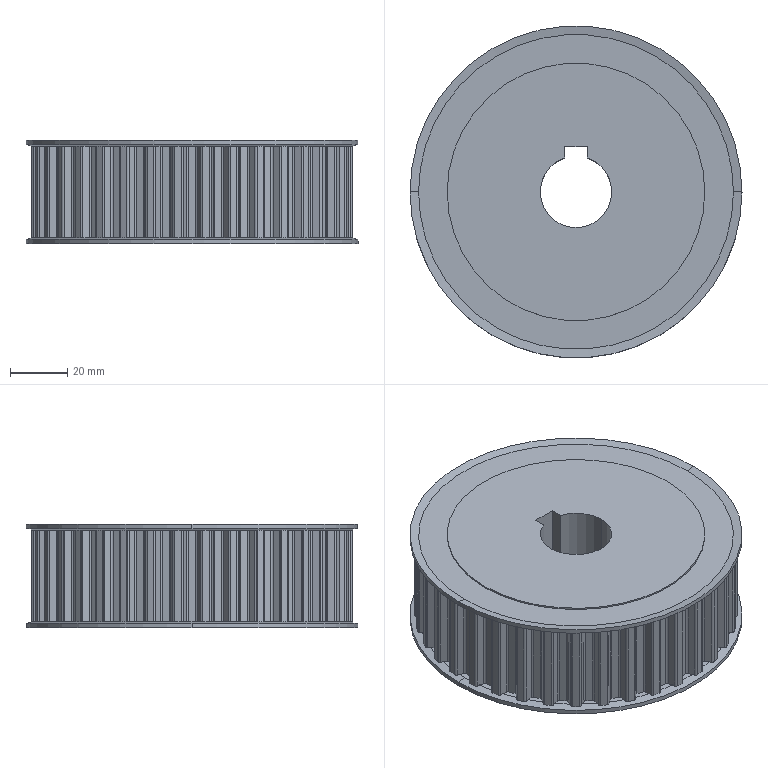Part | SolidWorks | features BaseBody 3 | 3 solids | 348 faces | box 116 x 116 x 36 mm | volume 319573 mm3 | cylinder 221 | plane 119 | cone 8 | commonest cylinder face diameters 1.6 x170 112.75 x36 90 x8 116 x4 25 x3